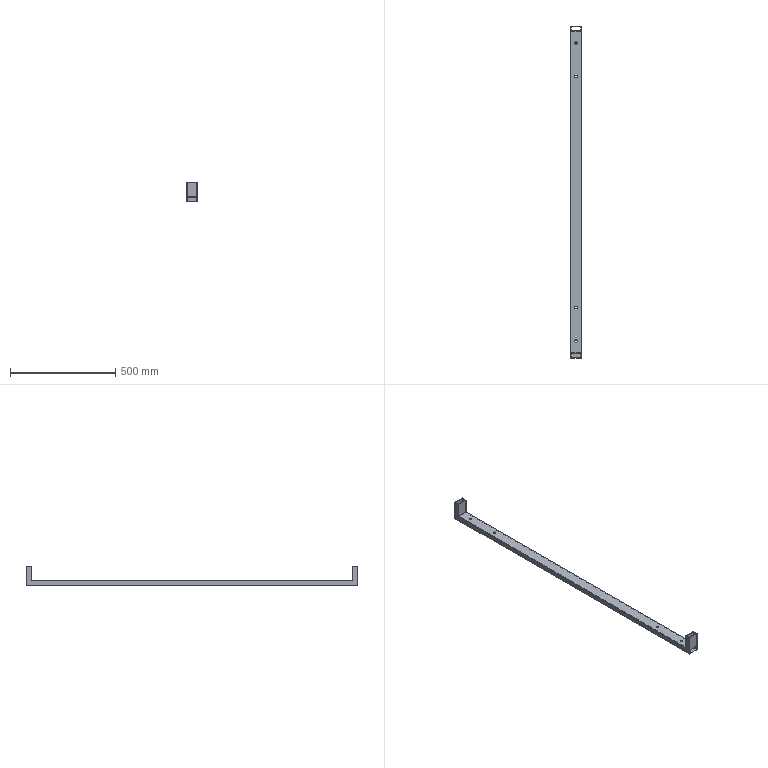Part | STEP file | ASND-0110-E63-HLTP01标准Lower机架-09 | 1 solid | 40 faces | box 50 x 1580 x 95 mm | volume 709366 mm3 | plane 24 | cylinder 16 | commonest cylinder face diameters 12 x16